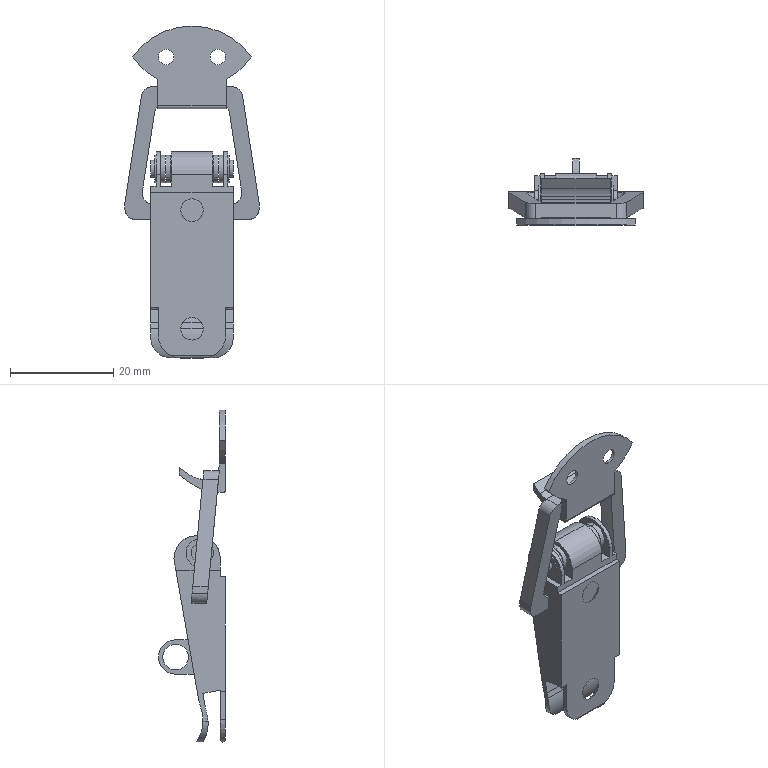Part | SolidWorks | features BaseBody 1 | 1 solid | 139 faces | box 26 x 13 x 64.364 mm | volume 4721 mm3 | plane 66 | cylinder 65 | cone 8 | commonest cylinder face diameters 5.333 x12 0.2 x8 3.333 x8 4 x8 9 x5 3 x4